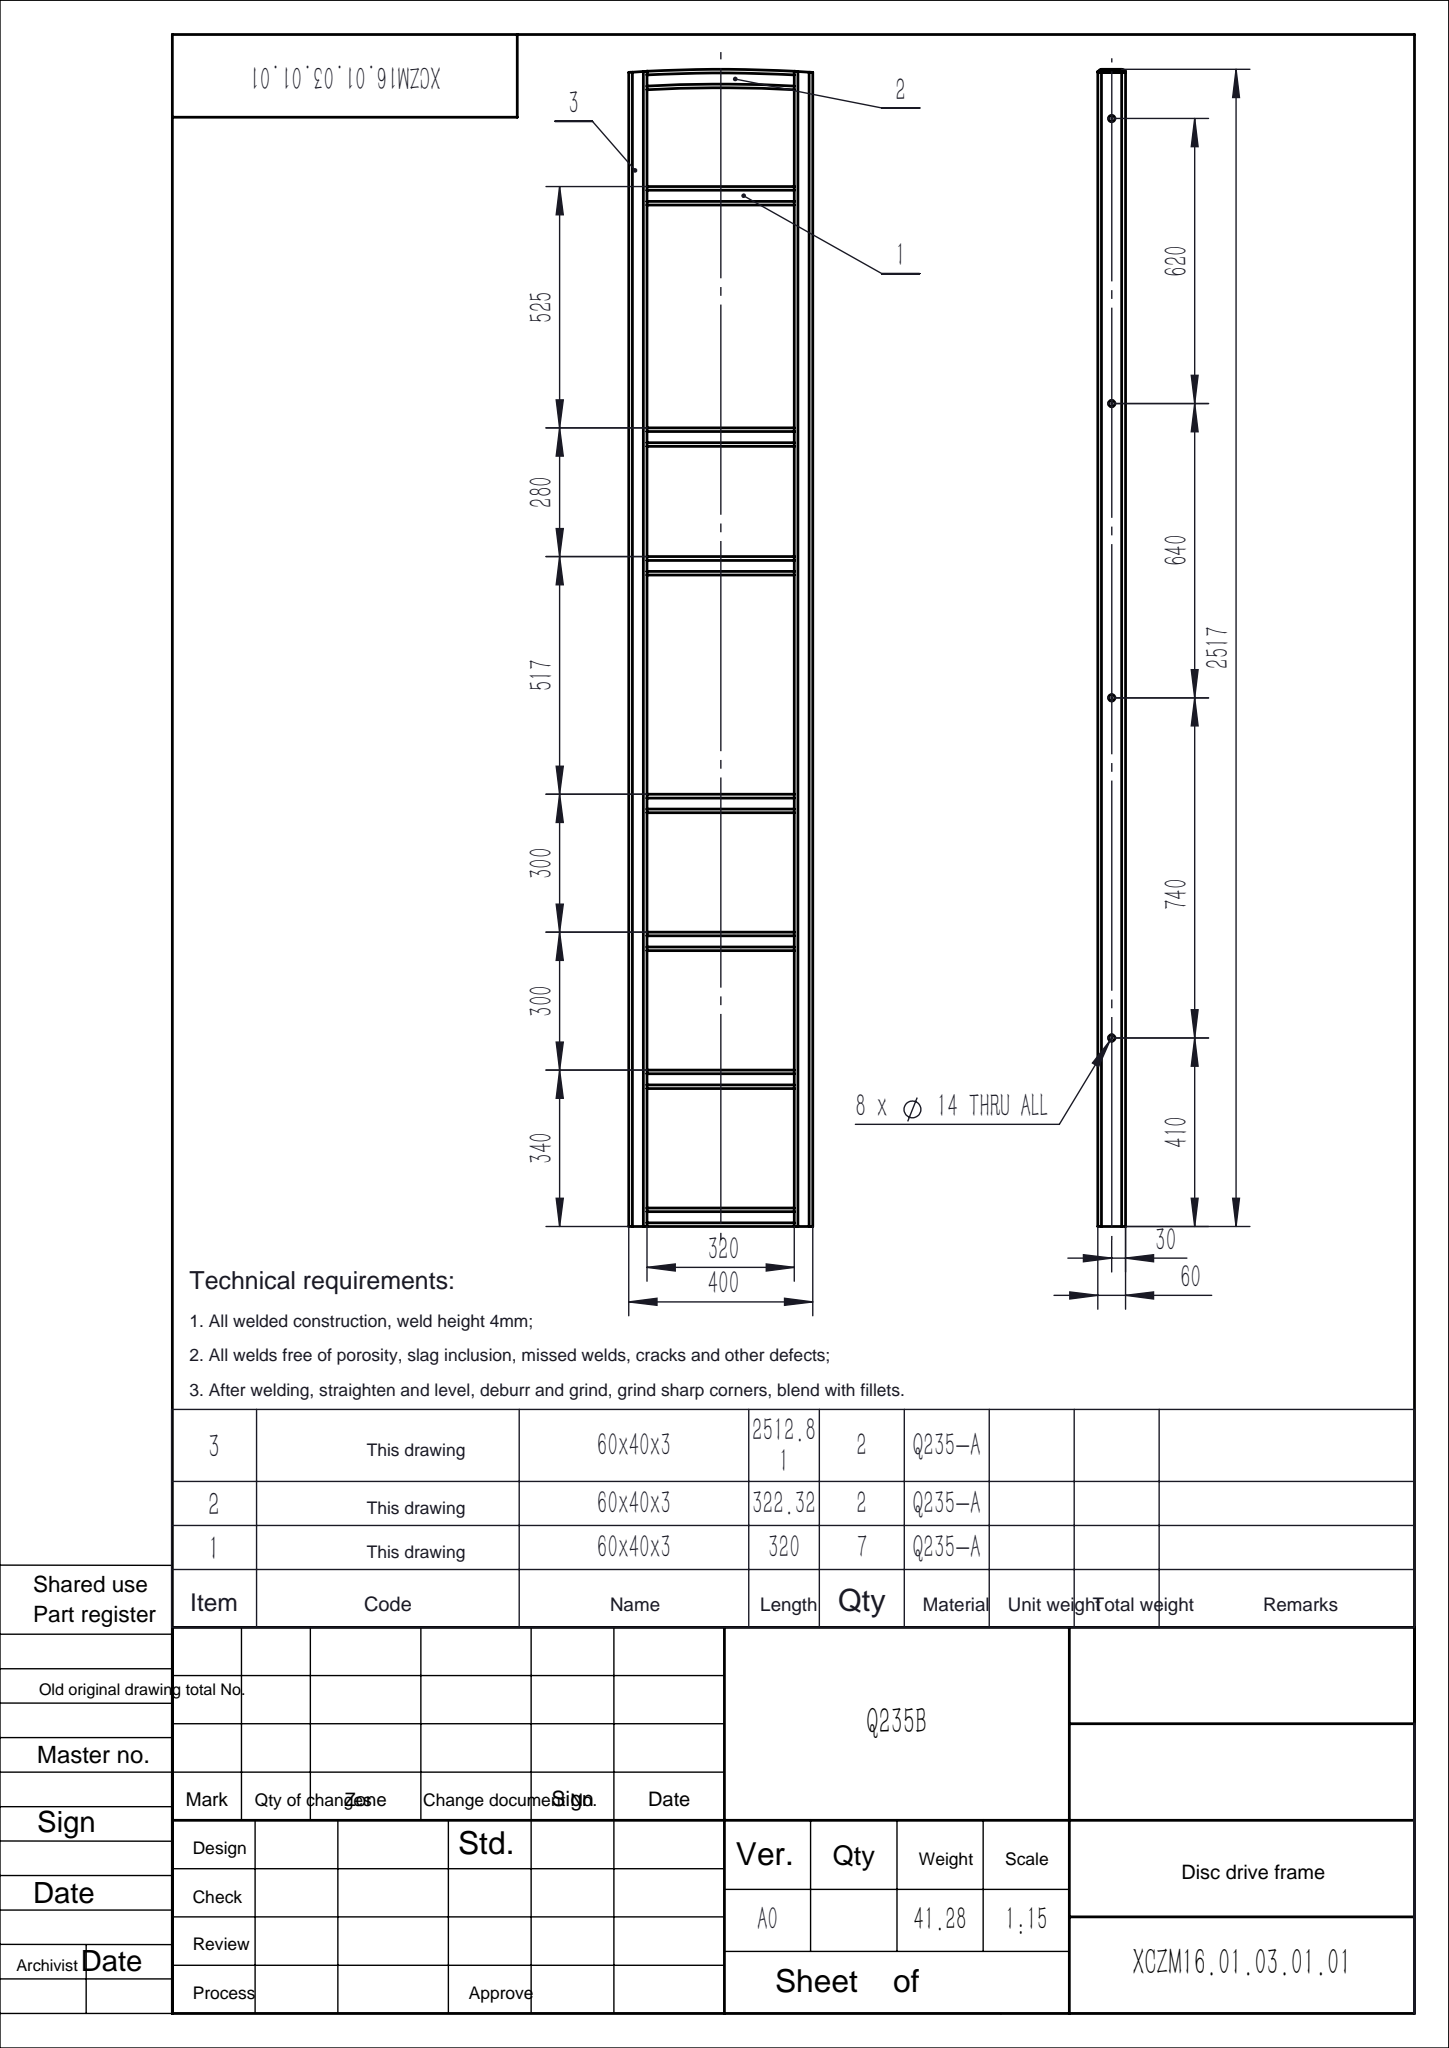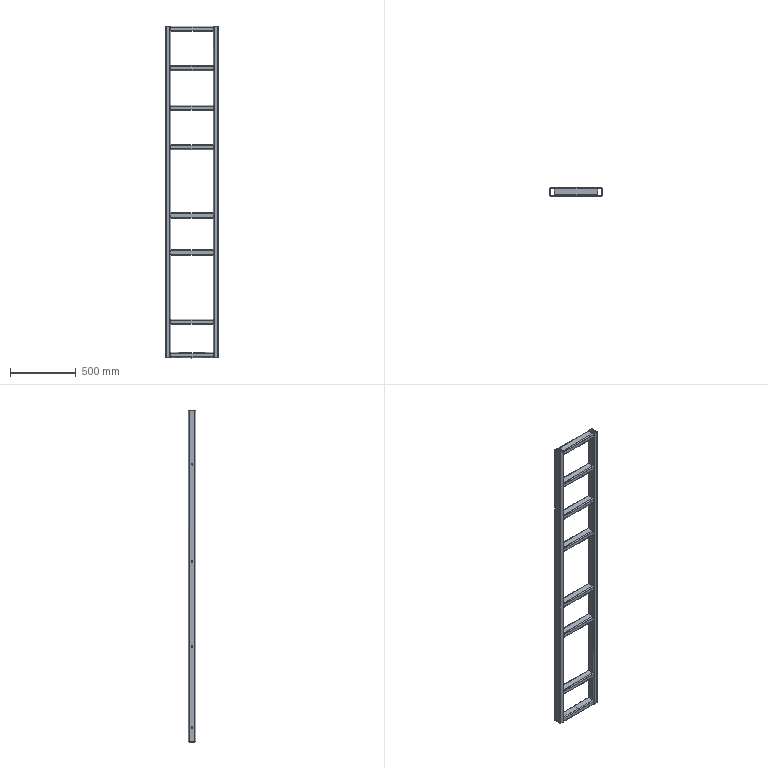Part | SolidWorks | features HoleWzd 1, WeldMemberFeat 1, WeldmentFeature 1 | 10 solids | 224 faces | box 400 x 60 x 2517 mm | volume 5259030 mm3 | cylinder 112 | plane 96 | torus 16 | commonest cylinder face diameters 8 x36 16 x36 14 x32 5920 x2 5928 x2 5992 x2